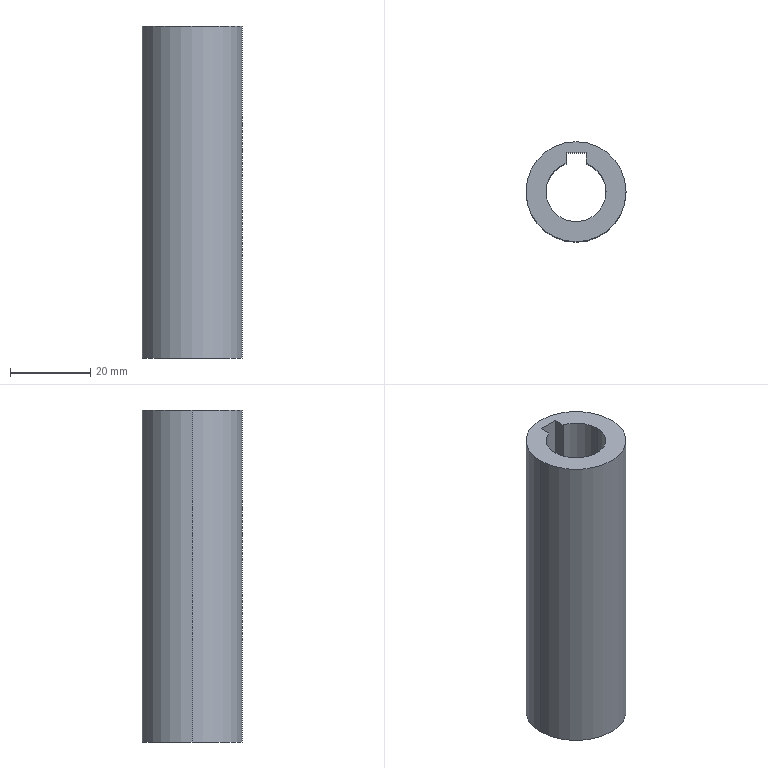Part | STEP file | 0228_Z_Gearhead_5GN120RH2 | 1 solid | 10 faces | box 25 x 25 x 83 mm | volume 25062 mm3 | cylinder 5 | plane 5 | commonest cylinder face diameters 15 x3 25 x2
STEP:
#1=CARTESIAN_POINT('',(0.,0.,0.));
#2=DIRECTION('',(0.,0.,1.));
#3=DIRECTION('',(1.,0.,0.));
#4=AXIS2_PLACEMENT_3D('',#1,#2,#3);
#5=CARTESIAN_POINT('',(7.5,0.,-83.));
#6=VERTEX_POINT('',#5);
#7=CARTESIAN_POINT('',(7.5,0.,0.));
#8=VERTEX_POINT('',#7);
#9=CARTESIAN_POINT('',(7.5,0.,22.109));
#10=DIRECTION('',(0.,0.,1.));
#11=VECTOR('',#10,1.);
#12=LINE('',#9,#11);
#13=CARTESIAN_POINT('',(0.,0.,22.109));
#14=DIRECTION('',(0.,0.,1.));
#15=DIRECTION('',(1.,0.,0.));
#16=AXIS2_PLACEMENT_3D('',#13,#14,#15);
#17=CYLINDRICAL_SURFACE('',#16,7.5);
#18=CARTESIAN_POINT('',(6.283,0.));
#19=DIRECTION('',(0.,1.));
#20=VECTOR('',#19,1.);
#21=LINE('',#18,#20);
#22=(GEOMETRIC_REPRESENTATION_CONTEXT(2)PARAMETRIC_REPRESENTATION_CONTEXT()REPRESENTATION_CONTEXT('',''));
#23=DEFINITIONAL_REPRESENTATION('',(#21),#22);
#24=PCURVE('',#17,#23);
#25=CARTESIAN_POINT('',(0.,0.,22.109));
#26=DIRECTION('',(0.,0.,1.));
#27=DIRECTION('',(1.,0.,0.));
#28=AXIS2_PLACEMENT_3D('',#25,#26,#27);
#29=CYLINDRICAL_SURFACE('',#28,7.5);
#30=CARTESIAN_POINT('',(0.,0.));
#31=DIRECTION('',(0.,1.));
#32=VECTOR('',#31,1.);
#33=LINE('',#30,#32);
#34=(GEOMETRIC_REPRESENTATION_CONTEXT(2)PARAMETRIC_REPRESENTATION_CONTEXT()REPRESENTATION_CONTEXT('',''));
#35=DEFINITIONAL_REPRESENTATION('',(#33),#34);
#36=PCURVE('',#29,#35);
#37=SURFACE_CURVE('',#12,(#24,#36),.PCURVE_S1.);
#38=EDGE_CURVE('',#6,#8,#37,.T.);
#39=ORIENTED_EDGE('',*,*,#38,.T.);
#40=CARTESIAN_POINT('',(-7.5,0.,0.));
#41=VERTEX_POINT('',#40);
#42=CARTESIAN_POINT('',(0.,0.,0.));
#43=DIRECTION('',(0.,0.,1.));
#44=DIRECTION('',(1.,0.,0.));
#45=AXIS2_PLACEMENT_3D('',#42,#43,#44);
#46=CIRCLE('',#45,7.5);
#47=CARTESIAN_POINT('',(0.,-22.109));
#48=DIRECTION('',(1.,0.));
#49=VECTOR('',#48,1.);
#50=LINE('',#47,#49);
#51=(GEOMETRIC_REPRESENTATION_CONTEXT(2)PARAMETRIC_REPRESENTATION_CONTEXT()REPRESENTATION_CONTEXT('',''));
#52=DEFINITIONAL_REPRESENTATION('',(#50),#51);
#53=PCURVE('',#17,#52);
#54=CARTESIAN_POINT('',(0.,0.,0.));
#55=DIRECTION('',(0.,0.,-1.));
#56=DIRECTION('',(-1.,0.,0.));
#57=AXIS2_PLACEMENT_3D('',#54,#55,#56);
#58=PLANE('',#57);
#59=CARTESIAN_POINT('',(-7.5,0.));
#60=CARTESIAN_POINT('',(-7.5,12.99));
#61=CARTESIAN_POINT('',(3.75,6.495));
#62=CARTESIAN_POINT('',(15.,0.));
#63=CARTESIAN_POINT('',(3.75,-6.495));
#64=CARTESIAN_POINT('',(-7.5,-12.99));
#65=CARTESIAN_POINT('',(-7.5,0.));
#66=(BOUNDED_CURVE()B_SPLINE_CURVE(2,(#59,#60,#61,#62,#63,#64,#65),.UNSPECIFIED.,.T.,.F.)B_SPLINE_CURVE_WITH_KNOTS((1,2,2,2,2,1),(-2.094,0.,2.094,4.189,6.283,8.378),.UNSPECIFIED.)CURVE()GEOMETRIC_REPRESENTATION_ITEM()RATIONAL_B_SPLINE_CURVE((1.,0.5,1.,0.5,1.,0.5,1.))REPRESENTATION_ITEM(''));
#67=(GEOMETRIC_REPRESENTATION_CONTEXT(2)PARAMETRIC_REPRESENTATION_CONTEXT()REPRESENTATION_CONTEXT('',''));
#68=DEFINITIONAL_REPRESENTATION('',(#66),#67);
#69=PCURVE('',#58,#68);
#70=SURFACE_CURVE('',#46,(#53,#69),.PCURVE_S1.);
#71=EDGE_CURVE('',#41,#8,#70,.T.);
#72=ORIENTED_EDGE('',*,*,#71,.F.);
#73=CARTESIAN_POINT('',(-7.5,0.,-83.));
#74=VERTEX_POINT('',#73);
#75=CARTESIAN_POINT('',(-7.5,0.,22.109));
#76=DIRECTION('',(0.,0.,1.));
#77=VECTOR('',#76,1.);
#78=LINE('',#75,#77);
#79=CARTESIAN_POINT('',(3.142,0.));
#80=DIRECTION('',(0.,1.));
#81=VECTOR('',#80,1.);
#82=LINE('',#79,#81);
#83=(GEOMETRIC_REPRESENTATION_CONTEXT(2)PARAMETRIC_REPRESENTATION_CONTEXT()REPRESENTATION_CONTEXT('',''));
#84=DEFINITIONAL_REPRESENTATION('',(#82),#83);
#85=PCURVE('',#17,#84);
#86=CARTESIAN_POINT('',(0.,0.,22.109));
#87=DIRECTION('',(0.,0.,1.));
#88=DIRECTION('',(1.,0.,0.));
#89=AXIS2_PLACEMENT_3D('',#86,#87,#88);
#90=CYLINDRICAL_SURFACE('',#89,7.5);
#91=CARTESIAN_POINT('',(3.142,0.));
#92=DIRECTION('',(0.,1.));
#93=VECTOR('',#92,1.);
#94=LINE('',#91,#93);
#95=(GEOMETRIC_REPRESENTATION_CONTEXT(2)PARAMETRIC_REPRESENTATION_CONTEXT()REPRESENTATION_CONTEXT('',''));
#96=DEFINITIONAL_REPRESENTATION('',(#94),#95);
#97=PCURVE('',#90,#96);
#98=SURFACE_CURVE('',#78,(#85,#97),.PCURVE_S1.);
#99=EDGE_CURVE('',#74,#41,#98,.T.);
#100=ORIENTED_EDGE('',*,*,#99,.F.);
#101=CARTESIAN_POINT('',(0.,0.,-83.));
#102=DIRECTION('',(0.,0.,1.));
#103=DIRECTION('',(1.,0.,0.));
#104=AXIS2_PLACEMENT_3D('',#101,#102,#103);
#105=CIRCLE('',#104,7.5);
#106=CARTESIAN_POINT('',(0.,-105.109));
#107=DIRECTION('',(1.,0.));
#108=VECTOR('',#107,1.);
#109=LINE('',#106,#108);
#110=(GEOMETRIC_REPRESENTATION_CONTEXT(2)PARAMETRIC_REPRESENTATION_CONTEXT()REPRESENTATION_CONTEXT('',''));
#111=DEFINITIONAL_REPRESENTATION('',(#109),#110);
#112=PCURVE('',#17,#111);
#113=CARTESIAN_POINT('',(0.,0.,-83.));
#114=DIRECTION('',(0.,0.,1.));
#115=DIRECTION('',(1.,0.,0.));
#116=AXIS2_PLACEMENT_3D('',#113,#114,#115);
#117=PLANE('',#116);
#118=CARTESIAN_POINT('',(0.,0.));
#119=DIRECTION('',(1.,0.));
#120=AXIS2_PLACEMENT_2D('',#118,#119);
#121=CIRCLE('',#120,7.5);
#122=(GEOMETRIC_REPRESENTATION_CONTEXT(2)PARAMETRIC_REPRESENTATION_CONTEXT()REPRESENTATION_CONTEXT('',''));
#123=DEFINITIONAL_REPRESENTATION('',(#121),#122);
#124=PCURVE('',#117,#123);
#125=SURFACE_CURVE('',#105,(#112,#124),.PCURVE_S1.);
#126=EDGE_CURVE('',#74,#6,#125,.T.);
#127=ORIENTED_EDGE('',*,*,#126,.T.);
#128=EDGE_LOOP('',(#39,#72,#100,#127));
#129=FACE_BOUND('',#128,.F.);
#130=ADVANCED_FACE('',(#129),#17,.F.);
#131=CARTESIAN_POINT('',(2.5,7.071,-83.));
#132=VERTEX_POINT('',#131);
#133=CARTESIAN_POINT('',(2.5,7.071,0.));
#134=VERTEX_POINT('',#133);
#135=CARTESIAN_POINT('',(2.5,7.071,-83.));
#136=DIRECTION('',(0.,0.,1.));
#137=VECTOR('',#136,1.);
#138=LINE('',#135,#137);
#139=CARTESIAN_POINT('',(1.231,-105.109));
#140=DIRECTION('',(0.,1.));
#141=VECTOR('',#140,1.);
#142=LINE('',#139,#141);
#143=(GEOMETRIC_REPRESENTATION_CONTEXT(2)PARAMETRIC_REPRESENTATION_CONTEXT()REPRESENTATION_CONTEXT('',''));
#144=DEFINITIONAL_REPRESENTATION('',(#142),#143);
#145=PCURVE('',#29,#144);
#146=CARTESIAN_POINT('',(2.5,9.8,-83.));
#147=DIRECTION('',(1.,0.,0.));
#148=DIRECTION('',(0.,1.,0.));
#149=AXIS2_PLACEMENT_3D('',#146,#147,#148);
#150=PLANE('',#149);
#151=CARTESIAN_POINT('',(-2.729,0.));
#152=DIRECTION('',(0.,1.));
#153=VECTOR('',#152,1.);
#154=LINE('',#151,#153);
#155=(GEOMETRIC_REPRESENTATION_CONTEXT(2)PARAMETRIC_REPRESENTATION_CONTEXT()REPRESENTATION_CONTEXT('',''));
#156=DEFINITIONAL_REPRESENTATION('',(#154),#155);
#157=PCURVE('',#150,#156);
#158=SURFACE_CURVE('',#138,(#145,#157),.PCURVE_S1.);
#159=EDGE_CURVE('',#132,#134,#158,.T.);
#160=ORIENTED_EDGE('',*,*,#159,.T.);
#161=CARTESIAN_POINT('',(0.,0.,0.));
#162=DIRECTION('',(0.,0.,1.));
#163=DIRECTION('',(1.,0.,0.));
#164=AXIS2_PLACEMENT_3D('',#161,#162,#163);
#165=CIRCLE('',#164,7.5);
#166=CARTESIAN_POINT('',(0.,-22.109));
#167=DIRECTION('',(1.,0.));
#168=VECTOR('',#167,1.);
#169=LINE('',#166,#168);
#170=(GEOMETRIC_REPRESENTATION_CONTEXT(2)PARAMETRIC_REPRESENTATION_CONTEXT()REPRESENTATION_CONTEXT('',''));
#171=DEFINITIONAL_REPRESENTATION('',(#169),#170);
#172=PCURVE('',#29,#171);
#173=CARTESIAN_POINT('',(-7.5,0.));
#174=CARTESIAN_POINT('',(-7.5,12.99));
#175=CARTESIAN_POINT('',(3.75,6.495));
#176=CARTESIAN_POINT('',(15.,0.));
#177=CARTESIAN_POINT('',(3.75,-6.495));
#178=CARTESIAN_POINT('',(-7.5,-12.99));
#179=CARTESIAN_POINT('',(-7.5,0.));
#180=(BOUNDED_CURVE()B_SPLINE_CURVE(2,(#173,#174,#175,#176,#177,#178,#179),.UNSPECIFIED.,.T.,.F.)B_SPLINE_CURVE_WITH_KNOTS((1,2,2,2,2,1),(-2.094,0.,2.094,4.189,6.283,8.378),.UNSPECIFIED.)CURVE()GEOMETRIC_REPRESENTATION_ITEM()RATIONAL_B_SPLINE_CURVE((1.,0.5,1.,0.5,1.,0.5,1.))REPRESENTATION_ITEM(''));
#181=(GEOMETRIC_REPRESENTATION_CONTEXT(2)PARAMETRIC_REPRESENTATION_CONTEXT()REPRESENTATION_CONTEXT('',''));
#182=DEFINITIONAL_REPRESENTATION('',(#180),#181);
#183=PCURVE('',#58,#182);
#184=SURFACE_CURVE('',#165,(#172,#183),.PCURVE_S1.);
#185=EDGE_CURVE('',#8,#134,#184,.T.);
#186=ORIENTED_EDGE('',*,*,#185,.F.);
#187=ORIENTED_EDGE('',*,*,#38,.F.);
#188=CARTESIAN_POINT('',(0.,0.,-83.));
#189=DIRECTION('',(0.,0.,1.));
#190=DIRECTION('',(1.,0.,0.));
#191=AXIS2_PLACEMENT_3D('',#188,#189,#190);
#192=CIRCLE('',#191,7.5);
#193=CARTESIAN_POINT('',(0.,-105.109));
#194=DIRECTION('',(1.,0.));
#195=VECTOR('',#194,1.);
#196=LINE('',#193,#195);
#197=(GEOMETRIC_REPRESENTATION_CONTEXT(2)PARAMETRIC_REPRESENTATION_CONTEXT()REPRESENTATION_CONTEXT('',''));
#198=DEFINITIONAL_REPRESENTATION('',(#196),#197);
#199=PCURVE('',#29,#198);
#200=CARTESIAN_POINT('',(0.,0.));
#201=DIRECTION('',(1.,0.));
#202=AXIS2_PLACEMENT_2D('',#200,#201);
#203=CIRCLE('',#202,7.5);
#204=(GEOMETRIC_REPRESENTATION_CONTEXT(2)PARAMETRIC_REPRESENTATION_CONTEXT()REPRESENTATION_CONTEXT('',''));
#205=DEFINITIONAL_REPRESENTATION('',(#203),#204);
#206=PCURVE('',#117,#205);
#207=SURFACE_CURVE('',#192,(#199,#206),.PCURVE_S1.);
#208=EDGE_CURVE('',#6,#132,#207,.T.);
#209=ORIENTED_EDGE('',*,*,#208,.T.);
#210=EDGE_LOOP('',(#160,#186,#187,#209));
#211=FACE_BOUND('',#210,.F.);
#212=ADVANCED_FACE('',(#211),#29,.F.);
#213=CARTESIAN_POINT('',(12.5,0.,-83.));
#214=VERTEX_POINT('',#213);
#215=CARTESIAN_POINT('',(-12.5,0.,-83.));
#216=VERTEX_POINT('',#215);
#217=CARTESIAN_POINT('',(0.,0.,-83.));
#218=DIRECTION('',(0.,0.,1.));
#219=DIRECTION('',(1.,0.,0.));
#220=AXIS2_PLACEMENT_3D('',#217,#218,#219);
#221=CIRCLE('',#220,12.5);
#222=CARTESIAN_POINT('',(0.,0.,11.169));
#223=DIRECTION('',(0.,0.,1.));
#224=DIRECTION('',(1.,0.,0.));
#225=AXIS2_PLACEMENT_3D('',#222,#223,#224);
#226=CYLINDRICAL_SURFACE('',#225,12.5);
#227=CARTESIAN_POINT('',(0.,-94.169));
#228=DIRECTION('',(1.,0.));
#229=VECTOR('',#228,1.);
#230=LINE('',#227,#229);
#231=(GEOMETRIC_REPRESENTATION_CONTEXT(2)PARAMETRIC_REPRESENTATION_CONTEXT()REPRESENTATION_CONTEXT('',''));
#232=DEFINITIONAL_REPRESENTATION('',(#230),#231);
#233=PCURVE('',#226,#232);
#234=CARTESIAN_POINT('',(0.,0.));
#235=DIRECTION('',(1.,0.));
#236=AXIS2_PLACEMENT_2D('',#234,#235);
#237=CIRCLE('',#236,12.5);
#238=(GEOMETRIC_REPRESENTATION_CONTEXT(2)PARAMETRIC_REPRESENTATION_CONTEXT()REPRESENTATION_CONTEXT('',''));
#239=DEFINITIONAL_REPRESENTATION('',(#237),#238);
#240=PCURVE('',#117,#239);
#241=SURFACE_CURVE('',#221,(#233,#240),.PCURVE_S1.);
#242=EDGE_CURVE('',#214,#216,#241,.T.);
#243=ORIENTED_EDGE('',*,*,#242,.T.);
#244=CARTESIAN_POINT('',(-12.5,0.,0.));
#245=VERTEX_POINT('',#244);
#246=CARTESIAN_POINT('',(-12.5,0.,11.169));
#247=DIRECTION('',(0.,0.,1.));
#248=VECTOR('',#247,1.);
#249=LINE('',#246,#248);
#250=CARTESIAN_POINT('',(3.142,0.));
#251=DIRECTION('',(0.,1.));
#252=VECTOR('',#251,1.);
#253=LINE('',#250,#252);
#254=(GEOMETRIC_REPRESENTATION_CONTEXT(2)PARAMETRIC_REPRESENTATION_CONTEXT()REPRESENTATION_CONTEXT('',''));
#255=DEFINITIONAL_REPRESENTATION('',(#253),#254);
#256=PCURVE('',#226,#255);
#257=CARTESIAN_POINT('',(0.,0.,11.169));
#258=DIRECTION('',(0.,0.,1.));
#259=DIRECTION('',(1.,0.,0.));
#260=AXIS2_PLACEMENT_3D('',#257,#258,#259);
#261=CYLINDRICAL_SURFACE('',#260,12.5);
#262=CARTESIAN_POINT('',(3.142,0.));
#263=DIRECTION('',(0.,1.));
#264=VECTOR('',#263,1.);
#265=LINE('',#262,#264);
#266=(GEOMETRIC_REPRESENTATION_CONTEXT(2)PARAMETRIC_REPRESENTATION_CONTEXT()REPRESENTATION_CONTEXT('',''));
#267=DEFINITIONAL_REPRESENTATION('',(#265),#266);
#268=PCURVE('',#261,#267);
#269=SURFACE_CURVE('',#249,(#256,#268),.PCURVE_S1.);
#270=EDGE_CURVE('',#216,#245,#269,.T.);
#271=ORIENTED_EDGE('',*,*,#270,.T.);
#272=CARTESIAN_POINT('',(12.5,0.,0.));
#273=VERTEX_POINT('',#272);
#274=CARTESIAN_POINT('',(0.,0.,0.));
#275=DIRECTION('',(0.,0.,1.));
#276=DIRECTION('',(1.,0.,0.));
#277=AXIS2_PLACEMENT_3D('',#274,#275,#276);
#278=CIRCLE('',#277,12.5);
#279=CARTESIAN_POINT('',(0.,-11.169));
#280=DIRECTION('',(1.,0.));
#281=VECTOR('',#280,1.);
#282=LINE('',#279,#281);
#283=(GEOMETRIC_REPRESENTATION_CONTEXT(2)PARAMETRIC_REPRESENTATION_CONTEXT()REPRESENTATION_CONTEXT('',''));
#284=DEFINITIONAL_REPRESENTATION('',(#282),#283);
#285=PCURVE('',#226,#284);
#286=CARTESIAN_POINT('',(-12.5,0.));
#287=CARTESIAN_POINT('',(-12.5,21.651));
#288=CARTESIAN_POINT('',(6.25,10.825));
#289=CARTESIAN_POINT('',(25.,0.));
#290=CARTESIAN_POINT('',(6.25,-10.825));
#291=CARTESIAN_POINT('',(-12.5,-21.651));
#292=CARTESIAN_POINT('',(-12.5,0.));
#293=(BOUNDED_CURVE()B_SPLINE_CURVE(2,(#286,#287,#288,#289,#290,#291,#292),.UNSPECIFIED.,.T.,.F.)B_SPLINE_CURVE_WITH_KNOTS((1,2,2,2,2,1),(-2.094,0.,2.094,4.189,6.283,8.378),.UNSPECIFIED.)CURVE()GEOMETRIC_REPRESENTATION_ITEM()RATIONAL_B_SPLINE_CURVE((1.,0.5,1.,0.5,1.,0.5,1.))REPRESENTATION_ITEM(''));
#294=(GEOMETRIC_REPRESENTATION_CONTEXT(2)PARAMETRIC_REPRESENTATION_CONTEXT()REPRESENTATION_CONTEXT('',''));
#295=DEFINITIONAL_REPRESENTATION('',(#293),#294);
#296=PCURVE('',#58,#295);
#297=SURFACE_CURVE('',#278,(#285,#296),.PCURVE_S1.);
#298=EDGE_CURVE('',#273,#245,#297,.T.);
#299=ORIENTED_EDGE('',*,*,#298,.F.);
#300=CARTESIAN_POINT('',(12.5,0.,11.169));
#301=DIRECTION('',(0.,0.,1.));
#302=VECTOR('',#301,1.);
#303=LINE('',#300,#302);
#304=CARTESIAN_POINT('',(0.,0.));
#305=DIRECTION('',(0.,1.));
#306=VECTOR('',#305,1.);
#307=LINE('',#304,#306);
#308=(GEOMETRIC_REPRESENTATION_CONTEXT(2)PARAMETRIC_REPRESENTATION_CONTEXT()REPRESENTATION_CONTEXT('',''));
#309=DEFINITIONAL_REPRESENTATION('',(#307),#308);
#310=PCURVE('',#226,#309);
#311=CARTESIAN_POINT('',(6.283,0.));
#312=DIRECTION('',(0.,1.));
#313=VECTOR('',#312,1.);
#314=LINE('',#311,#313);
#315=(GEOMETRIC_REPRESENTATION_CONTEXT(2)PARAMETRIC_REPRESENTATION_CONTEXT()REPRESENTATION_CONTEXT('',''));
#316=DEFINITIONAL_REPRESENTATION('',(#314),#315);
#317=PCURVE('',#261,#316);
#318=SURFACE_CURVE('',#303,(#310,#317),.PCURVE_S1.);
#319=EDGE_CURVE('',#214,#273,#318,.T.);
#320=ORIENTED_EDGE('',*,*,#319,.F.);
#321=EDGE_LOOP('',(#243,#271,#299,#320));
#322=FACE_BOUND('',#321,.T.);
#323=ADVANCED_FACE('',(#322),#226,.T.);
#324=ORIENTED_EDGE('',*,*,#298,.T.);
#325=CARTESIAN_POINT('',(0.,0.,0.));
#326=DIRECTION('',(0.,0.,1.));
#327=DIRECTION('',(1.,0.,0.));
#328=AXIS2_PLACEMENT_3D('',#325,#326,#327);
#329=CIRCLE('',#328,12.5);
#330=CARTESIAN_POINT('',(-12.5,0.));
#331=CARTESIAN_POINT('',(-12.5,21.651));
#332=CARTESIAN_POINT('',(6.25,10.825));
#333=CARTESIAN_POINT('',(25.,0.));
#334=CARTESIAN_POINT('',(6.25,-10.825));
#335=CARTESIAN_POINT('',(-12.5,-21.651));
#336=CARTESIAN_POINT('',(-12.5,0.));
#337=(BOUNDED_CURVE()B_SPLINE_CURVE(2,(#330,#331,#332,#333,#334,#335,#336),.UNSPECIFIED.,.T.,.F.)B_SPLINE_CURVE_WITH_KNOTS((1,2,2,2,2,1),(-2.094,0.,2.094,4.189,6.283,8.378),.UNSPECIFIED.)CURVE()GEOMETRIC_REPRESENTATION_ITEM()RATIONAL_B_SPLINE_CURVE((1.,0.5,1.,0.5,1.,0.5,1.))REPRESENTATION_ITEM(''));
#338=(GEOMETRIC_REPRESENTATION_CONTEXT(2)PARAMETRIC_REPRESENTATION_CONTEXT()REPRESENTATION_CONTEXT('',''));
#339=DEFINITIONAL_REPRESENTATION('',(#337),#338);
#340=PCURVE('',#58,#339);
#341=CARTESIAN_POINT('',(0.,-11.169));
#342=DIRECTION('',(1.,0.));
#343=VECTOR('',#342,1.);
#344=LINE('',#341,#343);
#345=(GEOMETRIC_REPRESENTATION_CONTEXT(2)PARAMETRIC_REPRESENTATION_CONTEXT()REPRESENTATION_CONTEXT('',''));
#346=DEFINITIONAL_REPRESENTATION('',(#344),#345);
#347=PCURVE('',#261,#346);
#348=SURFACE_CURVE('',#329,(#340,#347),.PCURVE_S1.);
#349=EDGE_CURVE('',#245,#273,#348,.T.);
#350=ORIENTED_EDGE('',*,*,#349,.T.);
#351=EDGE_LOOP('',(#324,#350));
#352=FACE_BOUND('',#351,.T.);
#353=CARTESIAN_POINT('',(-2.5,7.071,0.));
#354=VERTEX_POINT('',#353);
#355=CARTESIAN_POINT('',(0.,0.,0.));
#356=DIRECTION('',(0.,0.,1.));
#357=DIRECTION('',(1.,0.,0.));
#358=AXIS2_PLACEMENT_3D('',#355,#356,#357);
#359=CIRCLE('',#358,7.5);
#360=CARTESIAN_POINT('',(-7.5,0.));
#361=CARTESIAN_POINT('',(-7.5,12.99));
#362=CARTESIAN_POINT('',(3.75,6.495));
#363=CARTESIAN_POINT('',(15.,0.));
#364=CARTESIAN_POINT('',(3.75,-6.495));
#365=CARTESIAN_POINT('',(-7.5,-12.99));
#366=CARTESIAN_POINT('',(-7.5,0.));
#367=(BOUNDED_CURVE()B_SPLINE_CURVE(2,(#360,#361,#362,#363,#364,#365,#366),.UNSPECIFIED.,.T.,.F.)B_SPLINE_CURVE_WITH_KNOTS((1,2,2,2,2,1),(-2.094,0.,2.094,4.189,6.283,8.378),.UNSPECIFIED.)CURVE()GEOMETRIC_REPRESENTATION_ITEM()RATIONAL_B_SPLINE_CURVE((1.,0.5,1.,0.5,1.,0.5,1.))REPRESENTATION_ITEM(''));
#368=(GEOMETRIC_REPRESENTATION_CONTEXT(2)PARAMETRIC_REPRESENTATION_CONTEXT()REPRESENTATION_CONTEXT('',''));
#369=DEFINITIONAL_REPRESENTATION('',(#367),#368);
#370=PCURVE('',#58,#369);
#371=CARTESIAN_POINT('',(0.,-22.109));
#372=DIRECTION('',(1.,0.));
#373=VECTOR('',#372,1.);
#374=LINE('',#371,#373);
#375=(GEOMETRIC_REPRESENTATION_CONTEXT(2)PARAMETRIC_REPRESENTATION_CONTEXT()REPRESENTATION_CONTEXT('',''));
#376=DEFINITIONAL_REPRESENTATION('',(#374),#375);
#377=PCURVE('',#90,#376);
#378=SURFACE_CURVE('',#359,(#370,#377),.PCURVE_S1.);
#379=EDGE_CURVE('',#354,#41,#378,.T.);
#380=ORIENTED_EDGE('',*,*,#379,.F.);
#381=CARTESIAN_POINT('',(-2.5,9.8,0.));
#382=VERTEX_POINT('',#381);
#383=CARTESIAN_POINT('',(-2.5,9.8,0.));
#384=DIRECTION('',(0.,-1.,0.));
#385=VECTOR('',#384,1.);
#386=LINE('',#383,#385);
#387=CARTESIAN_POINT('',(2.5,9.8));
#388=DIRECTION('',(0.,-1.));
#389=VECTOR('',#388,1.);
#390=LINE('',#387,#389);
#391=(GEOMETRIC_REPRESENTATION_CONTEXT(2)PARAMETRIC_REPRESENTATION_CONTEXT()REPRESENTATION_CONTEXT('',''));
#392=DEFINITIONAL_REPRESENTATION('',(#390),#391);
#393=PCURVE('',#58,#392);
#394=CARTESIAN_POINT('',(-2.5,9.8,-83.));
#395=DIRECTION('',(-1.,0.,0.));
#396=DIRECTION('',(0.,-1.,0.));
#397=AXIS2_PLACEMENT_3D('',#394,#395,#396);
#398=PLANE('',#397);
#399=CARTESIAN_POINT('',(0.,83.));
#400=DIRECTION('',(1.,0.));
#401=VECTOR('',#400,1.);
#402=LINE('',#399,#401);
#403=(GEOMETRIC_REPRESENTATION_CONTEXT(2)PARAMETRIC_REPRESENTATION_CONTEXT()REPRESENTATION_CONTEXT('',''));
#404=DEFINITIONAL_REPRESENTATION('',(#402),#403);
#405=PCURVE('',#398,#404);
#406=SURFACE_CURVE('',#386,(#393,#405),.PCURVE_S1.);
#407=EDGE_CURVE('',#382,#354,#406,.T.);
#408=ORIENTED_EDGE('',*,*,#407,.F.);
#409=CARTESIAN_POINT('',(2.5,9.8,0.));
#410=VERTEX_POINT('',#409);
#411=CARTESIAN_POINT('',(-2.5,9.8,0.));
#412=DIRECTION('',(-1.,0.,0.));
#413=VECTOR('',#412,1.);
#414=LINE('',#411,#413);
#415=CARTESIAN_POINT('',(2.5,9.8));
#416=DIRECTION('',(1.,0.));
#417=VECTOR('',#416,1.);
#418=LINE('',#415,#417);
#419=(GEOMETRIC_REPRESENTATION_CONTEXT(2)PARAMETRIC_REPRESENTATION_CONTEXT()REPRESENTATION_CONTEXT('',''));
#420=DEFINITIONAL_REPRESENTATION('',(#418),#419);
#421=PCURVE('',#58,#420);
#422=CARTESIAN_POINT('',(-2.5,9.8,-83.));
#423=DIRECTION('',(0.,1.,0.));
#424=DIRECTION('',(0.,0.,1.));
#425=AXIS2_PLACEMENT_3D('',#422,#423,#424);
#426=PLANE('',#425);
#427=CARTESIAN_POINT('',(83.,0.));
#428=DIRECTION('',(0.,-1.));
#429=VECTOR('',#428,1.);
#430=LINE('',#427,#429);
#431=(GEOMETRIC_REPRESENTATION_CONTEXT(2)PARAMETRIC_REPRESENTATION_CONTEXT()REPRESENTATION_CONTEXT('',''));
#432=DEFINITIONAL_REPRESENTATION('',(#430),#431);
#433=PCURVE('',#426,#432);
#434=SURFACE_CURVE('',#414,(#421,#433),.PCURVE_S1.);
#435=EDGE_CURVE('',#410,#382,#434,.T.);
#436=ORIENTED_EDGE('',*,*,#435,.F.);
#437=CARTESIAN_POINT('',(2.5,9.8,0.));
#438=DIRECTION('',(0.,1.,0.));
#439=VECTOR('',#438,1.);
#440=LINE('',#437,#439);
#441=CARTESIAN_POINT('',(-2.5,9.8));
#442=DIRECTION('',(0.,1.));
#443=VECTOR('',#442,1.);
#444=LINE('',#441,#443);
#445=(GEOMETRIC_REPRESENTATION_CONTEXT(2)PARAMETRIC_REPRESENTATION_CONTEXT()REPRESENTATION_CONTEXT('',''));
#446=DEFINITIONAL_REPRESENTATION('',(#444),#445);
#447=PCURVE('',#58,#446);
#448=CARTESIAN_POINT('',(0.,83.));
#449=DIRECTION('',(1.,0.));
#450=VECTOR('',#449,1.);
#451=LINE('',#448,#450);
#452=(GEOMETRIC_REPRESENTATION_CONTEXT(2)PARAMETRIC_REPRESENTATION_CONTEXT()REPRESENTATION_CONTEXT('',''));
#453=DEFINITIONAL_REPRESENTATION('',(#451),#452);
#454=PCURVE('',#150,#453);
#455=SURFACE_CURVE('',#440,(#447,#454),.PCURVE_S1.);
#456=EDGE_CURVE('',#134,#410,#455,.T.);
#457=ORIENTED_EDGE('',*,*,#456,.F.);
#458=ORIENTED_EDGE('',*,*,#185,.F.);
#459=ORIENTED_EDGE('',*,*,#71,.F.);
#460=EDGE_LOOP('',(#380,#408,#436,#457,#458,#459));
#461=FACE_BOUND('',#460,.T.);
#462=ADVANCED_FACE('',(#352,#461),#58,.F.);
#463=ORIENTED_EDGE('',*,*,#242,.F.);
#464=CARTESIAN_POINT('',(0.,0.,-83.));
#465=DIRECTION('',(0.,0.,1.));
#466=DIRECTION('',(1.,0.,0.));
#467=AXIS2_PLACEMENT_3D('',#464,#465,#466);
#468=CIRCLE('',#467,12.5);
#469=CARTESIAN_POINT('',(0.,0.));
#470=DIRECTION('',(1.,0.));
#471=AXIS2_PLACEMENT_2D('',#469,#470);
#472=CIRCLE('',#471,12.5);
#473=(GEOMETRIC_REPRESENTATION_CONTEXT(2)PARAMETRIC_REPRESENTATION_CONTEXT()REPRESENTATION_CONTEXT('',''));
#474=DEFINITIONAL_REPRESENTATION('',(#472),#473);
#475=PCURVE('',#117,#474);
#476=CARTESIAN_POINT('',(0.,-94.169));
#477=DIRECTION('',(1.,0.));
#478=VECTOR('',#477,1.);
#479=LINE('',#476,#478);
#480=(GEOMETRIC_REPRESENTATION_CONTEXT(2)PARAMETRIC_REPRESENTATION_CONTEXT()REPRESENTATION_CONTEXT('',''));
#481=DEFINITIONAL_REPRESENTATION('',(#479),#480);
#482=PCURVE('',#261,#481);
#483=SURFACE_CURVE('',#468,(#475,#482),.PCURVE_S1.);
#484=EDGE_CURVE('',#216,#214,#483,.T.);
#485=ORIENTED_EDGE('',*,*,#484,.F.);
#486=EDGE_LOOP('',(#463,#485));
#487=FACE_BOUND('',#486,.T.);
#488=CARTESIAN_POINT('',(2.5,9.8,-83.));
#489=VERTEX_POINT('',#488);
#490=CARTESIAN_POINT('',(-2.5,9.8,-83.));
#491=VERTEX_POINT('',#490);
#492=CARTESIAN_POINT('',(-2.5,9.8,-83.));
#493=DIRECTION('',(-1.,0.,0.));
#494=VECTOR('',#493,1.);
#495=LINE('',#492,#494);
#496=CARTESIAN_POINT('',(-2.5,9.8));
#497=DIRECTION('',(-1.,0.));
#498=VECTOR('',#497,1.);
#499=LINE('',#496,#498);
#500=(GEOMETRIC_REPRESENTATION_CONTEXT(2)PARAMETRIC_REPRESENTATION_CONTEXT()REPRESENTATION_CONTEXT('',''));
#501=DEFINITIONAL_REPRESENTATION('',(#499),#500);
#502=PCURVE('',#117,#501);
#503=CARTESIAN_POINT('',(0.,0.));
#504=DIRECTION('',(0.,-1.));
#505=VECTOR('',#504,1.);
#506=LINE('',#503,#505);
#507=(GEOMETRIC_REPRESENTATION_CONTEXT(2)PARAMETRIC_REPRESENTATION_CONTEXT()REPRESENTATION_CONTEXT('',''));
#508=DEFINITIONAL_REPRESENTATION('',(#506),#507);
#509=PCURVE('',#426,#508);
#510=SURFACE_CURVE('',#495,(#502,#509),.PCURVE_S1.);
#511=EDGE_CURVE('',#489,#491,#510,.T.);
#512=ORIENTED_EDGE('',*,*,#511,.T.);
#513=CARTESIAN_POINT('',(-2.5,7.071,-83.));
#514=VERTEX_POINT('',#513);
#515=CARTESIAN_POINT('',(-2.5,9.8,-83.));
#516=DIRECTION('',(0.,-1.,0.));
#517=VECTOR('',#516,1.);
#518=LINE('',#515,#517);
#519=CARTESIAN_POINT('',(-2.5,9.8));
#520=DIRECTION('',(0.,-1.));
#521=VECTOR('',#520,1.);
#522=LINE('',#519,#521);
#523=(GEOMETRIC_REPRESENTATION_CONTEXT(2)PARAMETRIC_REPRESENTATION_CONTEXT()REPRESENTATION_CONTEXT('',''));
#524=DEFINITIONAL_REPRESENTATION('',(#522),#523);
#525=PCURVE('',#117,#524);
#526=CARTESIAN_POINT('',(0.,0.));
#527=DIRECTION('',(1.,0.));
#528=VECTOR('',#527,1.);
#529=LINE('',#526,#528);
#530=(GEOMETRIC_REPRESENTATION_CONTEXT(2)PARAMETRIC_REPRESENTATION_CONTEXT()REPRESENTATION_CONTEXT('',''));
#531=DEFINITIONAL_REPRESENTATION('',(#529),#530);
#532=PCURVE('',#398,#531);
#533=SURFACE_CURVE('',#518,(#525,#532),.PCURVE_S1.);
#534=EDGE_CURVE('',#491,#514,#533,.T.);
#535=ORIENTED_EDGE('',*,*,#534,.T.);
#536=CARTESIAN_POINT('',(0.,0.,-83.));
#537=DIRECTION('',(0.,0.,1.));
#538=DIRECTION('',(1.,0.,0.));
#539=AXIS2_PLACEMENT_3D('',#536,#537,#538);
#540=CIRCLE('',#539,7.5);
#541=CARTESIAN_POINT('',(0.,0.));
#542=DIRECTION('',(1.,0.));
#543=AXIS2_PLACEMENT_2D('',#541,#542);
#544=CIRCLE('',#543,7.5);
#545=(GEOMETRIC_REPRESENTATION_CONTEXT(2)PARAMETRIC_REPRESENTATION_CONTEXT()REPRESENTATION_CONTEXT('',''));
#546=DEFINITIONAL_REPRESENTATION('',(#544),#545);
#547=PCURVE('',#117,#546);
#548=CARTESIAN_POINT('',(0.,-105.109));
#549=DIRECTION('',(1.,0.));
#550=VECTOR('',#549,1.);
#551=LINE('',#548,#550);
#552=(GEOMETRIC_REPRESENTATION_CONTEXT(2)PARAMETRIC_REPRESENTATION_CONTEXT()REPRESENTATION_CONTEXT('',''));
#553=DEFINITIONAL_REPRESENTATION('',(#551),#552);
#554=PCURVE('',#90,#553);
#555=SURFACE_CURVE('',#540,(#547,#554),.PCURVE_S1.);
#556=EDGE_CURVE('',#514,#74,#555,.T.);
#557=ORIENTED_EDGE('',*,*,#556,.T.);
#558=ORIENTED_EDGE('',*,*,#126,.T.);
#559=ORIENTED_EDGE('',*,*,#208,.T.);
#560=CARTESIAN_POINT('',(2.5,9.8,-83.));
#561=DIRECTION('',(0.,1.,0.));
#562=VECTOR('',#561,1.);
#563=LINE('',#560,#562);
#564=CARTESIAN_POINT('',(2.5,9.8));
#565=DIRECTION('',(0.,1.));
#566=VECTOR('',#565,1.);
#567=LINE('',#564,#566);
#568=(GEOMETRIC_REPRESENTATION_CONTEXT(2)PARAMETRIC_REPRESENTATION_CONTEXT()REPRESENTATION_CONTEXT('',''));
#569=DEFINITIONAL_REPRESENTATION('',(#567),#568);
#570=PCURVE('',#117,#569);
#571=CARTESIAN_POINT('',(0.,0.));
#572=DIRECTION('',(1.,0.));
#573=VECTOR('',#572,1.);
#574=LINE('',#571,#573);
#575=(GEOMETRIC_REPRESENTATION_CONTEXT(2)PARAMETRIC_REPRESENTATION_CONTEXT()REPRESENTATION_CONTEXT('',''));
#576=DEFINITIONAL_REPRESENTATION('',(#574),#575);
#577=PCURVE('',#150,#576);
#578=SURFACE_CURVE('',#563,(#570,#577),.PCURVE_S1.);
#579=EDGE_CURVE('',#132,#489,#578,.T.);
#580=ORIENTED_EDGE('',*,*,#579,.T.);
#581=EDGE_LOOP('',(#512,#535,#557,#558,#559,#580));
#582=FACE_BOUND('',#581,.T.);
#583=ADVANCED_FACE('',(#487,#582),#117,.F.);
#584=ORIENTED_EDGE('',*,*,#270,.F.);
#585=ORIENTED_EDGE('',*,*,#484,.T.);
#586=ORIENTED_EDGE('',*,*,#319,.T.);
#587=ORIENTED_EDGE('',*,*,#349,.F.);
#588=EDGE_LOOP('',(#584,#585,#586,#587));
#589=FACE_BOUND('',#588,.T.);
#590=ADVANCED_FACE('',(#589),#261,.T.);
#591=ORIENTED_EDGE('',*,*,#379,.F.);
#592=CARTESIAN_POINT('',(-2.5,7.071,-83.));
#593=DIRECTION('',(0.,0.,1.));
#594=VECTOR('',#593,1.);
#595=LINE('',#592,#594);
#596=CARTESIAN_POINT('',(1.911,-105.109));
#597=DIRECTION('',(0.,1.));
#598=VECTOR('',#597,1.);
#599=LINE('',#596,#598);
#600=(GEOMETRIC_REPRESENTATION_CONTEXT(2)PARAMETRIC_REPRESENTATION_CONTEXT()REPRESENTATION_CONTEXT('',''));
#601=DEFINITIONAL_REPRESENTATION('',(#599),#600);
#602=PCURVE('',#90,#601);
#603=CARTESIAN_POINT('',(2.729,0.));
#604=DIRECTION('',(0.,1.));
#605=VECTOR('',#604,1.);
#606=LINE('',#603,#605);
#607=(GEOMETRIC_REPRESENTATION_CONTEXT(2)PARAMETRIC_REPRESENTATION_CONTEXT()REPRESENTATION_CONTEXT('',''));
#608=DEFINITIONAL_REPRESENTATION('',(#606),#607);
#609=PCURVE('',#398,#608);
#610=SURFACE_CURVE('',#595,(#602,#609),.PCURVE_S1.);
#611=EDGE_CURVE('',#514,#354,#610,.T.);
#612=ORIENTED_EDGE('',*,*,#611,.F.);
#613=ORIENTED_EDGE('',*,*,#556,.T.);
#614=ORIENTED_EDGE('',*,*,#99,.T.);
#615=EDGE_LOOP('',(#591,#612,#613,#614));
#616=FACE_BOUND('',#615,.F.);
#617=ADVANCED_FACE('',(#616),#90,.F.);
#618=ORIENTED_EDGE('',*,*,#407,.T.);
#619=ORIENTED_EDGE('',*,*,#611,.F.);
#620=ORIENTED_EDGE('',*,*,#534,.F.);
#621=CARTESIAN_POINT('',(-2.5,9.8,-83.));
#622=DIRECTION('',(0.,0.,1.));
#623=VECTOR('',#622,1.);
#624=LINE('',#621,#623);
#625=CARTESIAN_POINT('',(0.,0.));
#626=DIRECTION('',(0.,1.));
#627=VECTOR('',#626,1.);
#628=LINE('',#625,#627);
#629=(GEOMETRIC_REPRESENTATION_CONTEXT(2)PARAMETRIC_REPRESENTATION_CONTEXT()REPRESENTATION_CONTEXT('',''));
#630=DEFINITIONAL_REPRESENTATION('',(#628),#629);
#631=PCURVE('',#398,#630);
#632=CARTESIAN_POINT('',(0.,0.));
#633=DIRECTION('',(1.,0.));
#634=VECTOR('',#633,1.);
#635=LINE('',#632,#634);
#636=(GEOMETRIC_REPRESENTATION_CONTEXT(2)PARAMETRIC_REPRESENTATION_CONTEXT()REPRESENTATION_CONTEXT('',''));
#637=DEFINITIONAL_REPRESENTATION('',(#635),#636);
#638=PCURVE('',#426,#637);
#639=SURFACE_CURVE('',#624,(#631,#638),.PCURVE_S1.);
#640=EDGE_CURVE('',#491,#382,#639,.T.);
#641=ORIENTED_EDGE('',*,*,#640,.T.);
#642=EDGE_LOOP('',(#618,#619,#620,#641));
#643=FACE_BOUND('',#642,.T.);
#644=ADVANCED_FACE('',(#643),#398,.F.);
#645=ORIENTED_EDGE('',*,*,#435,.T.);
#646=ORIENTED_EDGE('',*,*,#640,.F.);
#647=ORIENTED_EDGE('',*,*,#511,.F.);
#648=CARTESIAN_POINT('',(2.5,9.8,-83.));
#649=DIRECTION('',(0.,0.,1.));
#650=VECTOR('',#649,1.);
#651=LINE('',#648,#650);
#652=CARTESIAN_POINT('',(0.,5.));
#653=DIRECTION('',(1.,0.));
#654=VECTOR('',#653,1.);
#655=LINE('',#652,#654);
#656=(GEOMETRIC_REPRESENTATION_CONTEXT(2)PARAMETRIC_REPRESENTATION_CONTEXT()REPRESENTATION_CONTEXT('',''));
#657=DEFINITIONAL_REPRESENTATION('',(#655),#656);
#658=PCURVE('',#426,#657);
#659=CARTESIAN_POINT('',(0.,0.));
#660=DIRECTION('',(0.,1.));
#661=VECTOR('',#660,1.);
#662=LINE('',#659,#661);
#663=(GEOMETRIC_REPRESENTATION_CONTEXT(2)PARAMETRIC_REPRESENTATION_CONTEXT()REPRESENTATION_CONTEXT('',''));
#664=DEFINITIONAL_REPRESENTATION('',(#662),#663);
#665=PCURVE('',#150,#664);
#666=SURFACE_CURVE('',#651,(#658,#665),.PCURVE_S1.);
#667=EDGE_CURVE('',#489,#410,#666,.T.);
#668=ORIENTED_EDGE('',*,*,#667,.T.);
#669=EDGE_LOOP('',(#645,#646,#647,#668));
#670=FACE_BOUND('',#669,.T.);
#671=ADVANCED_FACE('',(#670),#426,.F.);
#672=ORIENTED_EDGE('',*,*,#456,.T.);
#673=ORIENTED_EDGE('',*,*,#667,.F.);
#674=ORIENTED_EDGE('',*,*,#579,.F.);
#675=ORIENTED_EDGE('',*,*,#159,.T.);
#676=EDGE_LOOP('',(#672,#673,#674,#675));
#677=FACE_BOUND('',#676,.T.);
#678=ADVANCED_FACE('',(#677),#150,.F.);
#679=CLOSED_SHELL('',(#130,#212,#323,#462,#583,#590,#617,#644,#671,#678));
#680=MANIFOLD_SOLID_BREP('',#679);
#681=(LENGTH_UNIT()NAMED_UNIT(*)SI_UNIT(.MILLI.,.METRE.));
#682=UNCERTAINTY_MEASURE_WITH_UNIT(LENGTH_MEASURE(0.0000001),#681,'','');
#683=(NAMED_UNIT(*)PLANE_ANGLE_UNIT()SI_UNIT($,.RADIAN.));
#684=(NAMED_UNIT(*)SI_UNIT($,.STERADIAN.)SOLID_ANGLE_UNIT());
#685=(GEOMETRIC_REPRESENTATION_CONTEXT(3)GLOBAL_UNCERTAINTY_ASSIGNED_CONTEXT((#682))GLOBAL_UNIT_ASSIGNED_CONTEXT((#681,#683,#684))REPRESENTATION_CONTEXT('',''));
#686=ADVANCED_BREP_SHAPE_REPRESENTATION('',(#4,#680),#685);